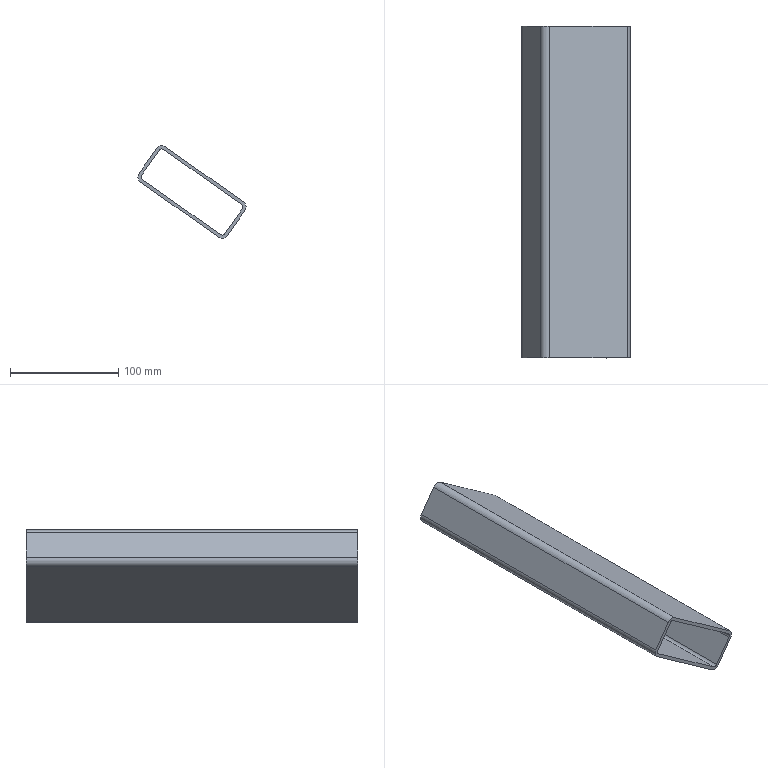Part | STEP file | new extension bracket | 1 solid | 18 faces | box 100.038 x 307.108 x 85.627 mm | volume 239797 mm3 | plane 10 | cylinder 8 | commonest cylinder face diameters 6 x4 12 x4
STEP:
#1=CARTESIAN_POINT('',(0.,0.,0.));
#2=DIRECTION('',(0.,0.,1.));
#3=DIRECTION('',(1.,0.,0.));
#4=AXIS2_PLACEMENT_3D('',#1,#2,#3);
#5=CARTESIAN_POINT('',(1487.978,118.392,730.631));
#6=VERTEX_POINT('',#5);
#7=CARTESIAN_POINT('',(1471.83,118.392,707.757));
#8=VERTEX_POINT('',#7);
#9=CARTESIAN_POINT('',(1489.709,118.392,733.082));
#10=DIRECTION('',(-0.5767,0.,-0.8169));
#11=VECTOR('',#10,1.);
#12=LINE('',#9,#11);
#13=CARTESIAN_POINT('',(0.,118.392,0.));
#14=DIRECTION('',(0.,1.,0.));
#15=DIRECTION('',(0.,0.,-1.));
#16=AXIS2_PLACEMENT_3D('',#13,#14,#15);
#17=PLANE('',#16);
#18=CARTESIAN_POINT('',(-733.082,-1489.709));
#19=DIRECTION('',(0.8169,0.5767));
#20=VECTOR('',#19,1.);
#21=LINE('',#18,#20);
#22=(GEOMETRIC_REPRESENTATION_CONTEXT(2)PARAMETRIC_REPRESENTATION_CONTEXT()REPRESENTATION_CONTEXT('',''));
#23=DEFINITIONAL_REPRESENTATION('',(#21),#22);
#24=PCURVE('',#17,#23);
#25=CARTESIAN_POINT('',(1489.709,425.5,733.082));
#26=DIRECTION('',(-0.8169,0.,0.5767));
#27=DIRECTION('',(-0.5767,0.,-0.8169));
#28=AXIS2_PLACEMENT_3D('',#25,#26,#27);
#29=PLANE('',#28);
#30=CARTESIAN_POINT('',(0.,307.108));
#31=DIRECTION('',(1.,0.));
#32=VECTOR('',#31,1.);
#33=LINE('',#30,#32);
#34=(GEOMETRIC_REPRESENTATION_CONTEXT(2)PARAMETRIC_REPRESENTATION_CONTEXT()REPRESENTATION_CONTEXT('',''));
#35=DEFINITIONAL_REPRESENTATION('',(#33),#34);
#36=PCURVE('',#29,#35);
#37=SURFACE_CURVE('',#12,(#24,#36),.PCURVE_S1.);
#38=EDGE_CURVE('',#6,#8,#37,.T.);
#39=ORIENTED_EDGE('',*,*,#38,.F.);
#40=CARTESIAN_POINT('',(1492.159,118.392,731.351));
#41=VERTEX_POINT('',#40);
#42=CARTESIAN_POINT('',(1490.429,118.392,728.901));
#43=DIRECTION('',(0.,1.,0.));
#44=DIRECTION('',(0.,0.,1.));
#45=AXIS2_PLACEMENT_3D('',#42,#43,#44);
#46=CIRCLE('',#45,3.);
#47=CARTESIAN_POINT('',(-728.901,-1490.429));
#48=DIRECTION('',(-1.,0.));
#49=AXIS2_PLACEMENT_2D('',#47,#48);
#50=CIRCLE('',#49,3.);
#51=(GEOMETRIC_REPRESENTATION_CONTEXT(2)PARAMETRIC_REPRESENTATION_CONTEXT()REPRESENTATION_CONTEXT('',''));
#52=DEFINITIONAL_REPRESENTATION('',(#50),#51);
#53=PCURVE('',#17,#52);
#54=CARTESIAN_POINT('',(1490.429,425.5,728.901));
#55=DIRECTION('',(0.,1.,0.));
#56=DIRECTION('',(1.,0.,0.));
#57=AXIS2_PLACEMENT_3D('',#54,#55,#56);
#58=CYLINDRICAL_SURFACE('',#57,3.);
#59=CARTESIAN_POINT('',(-1.571,-307.108));
#60=DIRECTION('',(1.,0.));
#61=VECTOR('',#60,1.);
#62=LINE('',#59,#61);
#63=(GEOMETRIC_REPRESENTATION_CONTEXT(2)PARAMETRIC_REPRESENTATION_CONTEXT()REPRESENTATION_CONTEXT('',''));
#64=DEFINITIONAL_REPRESENTATION('',(#62),#63);
#65=PCURVE('',#58,#64);
#66=SURFACE_CURVE('',#46,(#53,#65),.PCURVE_S1.);
#67=EDGE_CURVE('',#6,#41,#66,.T.);
#68=ORIENTED_EDGE('',*,*,#67,.T.);
#69=CARTESIAN_POINT('',(1564.049,118.392,680.598));
#70=VERTEX_POINT('',#69);
#71=CARTESIAN_POINT('',(1566.5,118.392,678.868));
#72=DIRECTION('',(-0.8169,0.,0.5767));
#73=VECTOR('',#72,1.);
#74=LINE('',#71,#73);
#75=CARTESIAN_POINT('',(-678.868,-1566.5));
#76=DIRECTION('',(-0.5767,0.8169));
#77=VECTOR('',#76,1.);
#78=LINE('',#75,#77);
#79=(GEOMETRIC_REPRESENTATION_CONTEXT(2)PARAMETRIC_REPRESENTATION_CONTEXT()REPRESENTATION_CONTEXT('',''));
#80=DEFINITIONAL_REPRESENTATION('',(#78),#79);
#81=PCURVE('',#17,#80);
#82=CARTESIAN_POINT('',(1566.5,425.5,678.868));
#83=DIRECTION('',(0.5767,0.,0.8169));
#84=DIRECTION('',(-0.8169,0.,0.5767));
#85=AXIS2_PLACEMENT_3D('',#82,#83,#84);
#86=PLANE('',#85);
#87=CARTESIAN_POINT('',(0.,307.108));
#88=DIRECTION('',(1.,0.));
#89=VECTOR('',#88,1.);
#90=LINE('',#87,#89);
#91=(GEOMETRIC_REPRESENTATION_CONTEXT(2)PARAMETRIC_REPRESENTATION_CONTEXT()REPRESENTATION_CONTEXT('',''));
#92=DEFINITIONAL_REPRESENTATION('',(#90),#91);
#93=PCURVE('',#86,#92);
#94=SURFACE_CURVE('',#74,(#81,#93),.PCURVE_S1.);
#95=EDGE_CURVE('',#70,#41,#94,.T.);
#96=ORIENTED_EDGE('',*,*,#95,.F.);
#97=CARTESIAN_POINT('',(1564.77,118.392,676.417));
#98=VERTEX_POINT('',#97);
#99=CARTESIAN_POINT('',(1562.319,118.392,678.148));
#100=DIRECTION('',(0.,1.,0.));
#101=DIRECTION('',(0.,0.,1.));
#102=AXIS2_PLACEMENT_3D('',#99,#100,#101);
#103=CIRCLE('',#102,3.);
#104=CARTESIAN_POINT('',(-678.148,-1562.319));
#105=DIRECTION('',(-1.,0.));
#106=AXIS2_PLACEMENT_2D('',#104,#105);
#107=CIRCLE('',#106,3.);
#108=(GEOMETRIC_REPRESENTATION_CONTEXT(2)PARAMETRIC_REPRESENTATION_CONTEXT()REPRESENTATION_CONTEXT('',''));
#109=DEFINITIONAL_REPRESENTATION('',(#107),#108);
#110=PCURVE('',#17,#109);
#111=CARTESIAN_POINT('',(1562.319,425.5,678.148));
#112=DIRECTION('',(0.,1.,0.));
#113=DIRECTION('',(1.,0.,0.));
#114=AXIS2_PLACEMENT_3D('',#111,#112,#113);
#115=CYLINDRICAL_SURFACE('',#114,3.);
#116=CARTESIAN_POINT('',(4.712,-307.108));
#117=DIRECTION('',(1.,0.));
#118=VECTOR('',#117,1.);
#119=LINE('',#116,#118);
#120=(GEOMETRIC_REPRESENTATION_CONTEXT(2)PARAMETRIC_REPRESENTATION_CONTEXT()REPRESENTATION_CONTEXT('',''));
#121=DEFINITIONAL_REPRESENTATION('',(#119),#120);
#122=PCURVE('',#115,#121);
#123=SURFACE_CURVE('',#103,(#110,#122),.PCURVE_S1.);
#124=EDGE_CURVE('',#70,#98,#123,.T.);
#125=ORIENTED_EDGE('',*,*,#124,.T.);
#126=CARTESIAN_POINT('',(1548.621,118.392,653.543));
#127=VERTEX_POINT('',#126);
#128=CARTESIAN_POINT('',(1546.891,118.392,651.093));
#129=DIRECTION('',(0.5767,0.,0.8169));
#130=VECTOR('',#129,1.);
#131=LINE('',#128,#130);
#132=CARTESIAN_POINT('',(-651.093,-1546.891));
#133=DIRECTION('',(-0.8169,-0.5767));
#134=VECTOR('',#133,1.);
#135=LINE('',#132,#134);
#136=(GEOMETRIC_REPRESENTATION_CONTEXT(2)PARAMETRIC_REPRESENTATION_CONTEXT()REPRESENTATION_CONTEXT('',''));
#137=DEFINITIONAL_REPRESENTATION('',(#135),#136);
#138=PCURVE('',#17,#137);
#139=CARTESIAN_POINT('',(1546.891,425.5,651.093));
#140=DIRECTION('',(0.8169,0.,-0.5767));
#141=DIRECTION('',(0.5767,0.,0.8169));
#142=AXIS2_PLACEMENT_3D('',#139,#140,#141);
#143=PLANE('',#142);
#144=CARTESIAN_POINT('',(0.,307.108));
#145=DIRECTION('',(1.,0.));
#146=VECTOR('',#145,1.);
#147=LINE('',#144,#146);
#148=(GEOMETRIC_REPRESENTATION_CONTEXT(2)PARAMETRIC_REPRESENTATION_CONTEXT()REPRESENTATION_CONTEXT('',''));
#149=DEFINITIONAL_REPRESENTATION('',(#147),#148);
#150=PCURVE('',#143,#149);
#151=SURFACE_CURVE('',#131,(#138,#150),.PCURVE_S1.);
#152=EDGE_CURVE('',#127,#98,#151,.T.);
#153=ORIENTED_EDGE('',*,*,#152,.F.);
#154=CARTESIAN_POINT('',(1544.44,118.392,652.823));
#155=VERTEX_POINT('',#154);
#156=CARTESIAN_POINT('',(1546.17,118.392,655.274));
#157=DIRECTION('',(0.,1.,0.));
#158=DIRECTION('',(0.,0.,1.));
#159=AXIS2_PLACEMENT_3D('',#156,#157,#158);
#160=CIRCLE('',#159,3.);
#161=CARTESIAN_POINT('',(-655.274,-1546.17));
#162=DIRECTION('',(-1.,0.));
#163=AXIS2_PLACEMENT_2D('',#161,#162);
#164=CIRCLE('',#163,3.);
#165=(GEOMETRIC_REPRESENTATION_CONTEXT(2)PARAMETRIC_REPRESENTATION_CONTEXT()REPRESENTATION_CONTEXT('',''));
#166=DEFINITIONAL_REPRESENTATION('',(#164),#165);
#167=PCURVE('',#17,#166);
#168=CARTESIAN_POINT('',(1546.17,425.5,655.274));
#169=DIRECTION('',(0.,1.,0.));
#170=DIRECTION('',(1.,0.,0.));
#171=AXIS2_PLACEMENT_3D('',#168,#169,#170);
#172=CYLINDRICAL_SURFACE('',#171,3.);
#173=CARTESIAN_POINT('',(-1.571,-307.108));
#174=DIRECTION('',(1.,0.));
#175=VECTOR('',#174,1.);
#176=LINE('',#173,#175);
#177=(GEOMETRIC_REPRESENTATION_CONTEXT(2)PARAMETRIC_REPRESENTATION_CONTEXT()REPRESENTATION_CONTEXT('',''));
#178=DEFINITIONAL_REPRESENTATION('',(#176),#177);
#179=PCURVE('',#172,#178);
#180=SURFACE_CURVE('',#160,(#167,#179),.PCURVE_S1.);
#181=EDGE_CURVE('',#127,#155,#180,.T.);
#182=ORIENTED_EDGE('',*,*,#181,.T.);
#183=CARTESIAN_POINT('',(1472.55,118.392,703.576));
#184=VERTEX_POINT('',#183);
#185=CARTESIAN_POINT('',(1470.099,118.392,705.306));
#186=DIRECTION('',(0.8169,0.,-0.5767));
#187=VECTOR('',#186,1.);
#188=LINE('',#185,#187);
#189=CARTESIAN_POINT('',(-705.306,-1470.099));
#190=DIRECTION('',(0.5767,-0.8169));
#191=VECTOR('',#190,1.);
#192=LINE('',#189,#191);
#193=(GEOMETRIC_REPRESENTATION_CONTEXT(2)PARAMETRIC_REPRESENTATION_CONTEXT()REPRESENTATION_CONTEXT('',''));
#194=DEFINITIONAL_REPRESENTATION('',(#192),#193);
#195=PCURVE('',#17,#194);
#196=CARTESIAN_POINT('',(1470.099,425.5,705.306));
#197=DIRECTION('',(-0.5767,0.,-0.8169));
#198=DIRECTION('',(0.8169,0.,-0.5767));
#199=AXIS2_PLACEMENT_3D('',#196,#197,#198);
#200=PLANE('',#199);
#201=CARTESIAN_POINT('',(0.,307.108));
#202=DIRECTION('',(1.,0.));
#203=VECTOR('',#202,1.);
#204=LINE('',#201,#203);
#205=(GEOMETRIC_REPRESENTATION_CONTEXT(2)PARAMETRIC_REPRESENTATION_CONTEXT()REPRESENTATION_CONTEXT('',''));
#206=DEFINITIONAL_REPRESENTATION('',(#204),#205);
#207=PCURVE('',#200,#206);
#208=SURFACE_CURVE('',#188,(#195,#207),.PCURVE_S1.);
#209=EDGE_CURVE('',#184,#155,#208,.T.);
#210=ORIENTED_EDGE('',*,*,#209,.F.);
#211=CARTESIAN_POINT('',(1474.28,118.392,706.027));
#212=DIRECTION('',(0.,1.,0.));
#213=DIRECTION('',(0.,0.,1.));
#214=AXIS2_PLACEMENT_3D('',#211,#212,#213);
#215=CIRCLE('',#214,3.);
#216=CARTESIAN_POINT('',(-706.027,-1474.28));
#217=DIRECTION('',(-1.,0.));
#218=AXIS2_PLACEMENT_2D('',#216,#217);
#219=CIRCLE('',#218,3.);
#220=(GEOMETRIC_REPRESENTATION_CONTEXT(2)PARAMETRIC_REPRESENTATION_CONTEXT()REPRESENTATION_CONTEXT('',''));
#221=DEFINITIONAL_REPRESENTATION('',(#219),#220);
#222=PCURVE('',#17,#221);
#223=CARTESIAN_POINT('',(1474.28,425.5,706.027));
#224=DIRECTION('',(0.,1.,0.));
#225=DIRECTION('',(1.,0.,0.));
#226=AXIS2_PLACEMENT_3D('',#223,#224,#225);
#227=CYLINDRICAL_SURFACE('',#226,3.);
#228=CARTESIAN_POINT('',(-1.571,-307.108));
#229=DIRECTION('',(1.,0.));
#230=VECTOR('',#229,1.);
#231=LINE('',#228,#230);
#232=(GEOMETRIC_REPRESENTATION_CONTEXT(2)PARAMETRIC_REPRESENTATION_CONTEXT()REPRESENTATION_CONTEXT('',''));
#233=DEFINITIONAL_REPRESENTATION('',(#231),#232);
#234=PCURVE('',#227,#233);
#235=SURFACE_CURVE('',#215,(#222,#234),.PCURVE_S1.);
#236=EDGE_CURVE('',#184,#8,#235,.T.);
#237=ORIENTED_EDGE('',*,*,#236,.T.);
#238=EDGE_LOOP('',(#39,#68,#96,#125,#153,#182,#210,#237));
#239=FACE_BOUND('',#238,.T.);
#240=CARTESIAN_POINT('',(1542.71,118.392,650.372));
#241=VERTEX_POINT('',#240);
#242=CARTESIAN_POINT('',(1470.82,118.392,701.125));
#243=VERTEX_POINT('',#242);
#244=CARTESIAN_POINT('',(1547.611,118.392,646.912));
#245=DIRECTION('',(-0.8169,0.,0.5767));
#246=VECTOR('',#245,1.);
#247=LINE('',#244,#246);
#248=CARTESIAN_POINT('',(-646.912,-1547.611));
#249=DIRECTION('',(-0.5767,0.8169));
#250=VECTOR('',#249,1.);
#251=LINE('',#248,#250);
#252=(GEOMETRIC_REPRESENTATION_CONTEXT(2)PARAMETRIC_REPRESENTATION_CONTEXT()REPRESENTATION_CONTEXT('',''));
#253=DEFINITIONAL_REPRESENTATION('',(#251),#252);
#254=PCURVE('',#17,#253);
#255=CARTESIAN_POINT('',(1547.611,425.5,646.912));
#256=DIRECTION('',(0.5767,0.,0.8169));
#257=DIRECTION('',(-0.8169,0.,0.5767));
#258=AXIS2_PLACEMENT_3D('',#255,#256,#257);
#259=PLANE('',#258);
#260=CARTESIAN_POINT('',(0.,307.108));
#261=DIRECTION('',(1.,0.));
#262=VECTOR('',#261,1.);
#263=LINE('',#260,#262);
#264=(GEOMETRIC_REPRESENTATION_CONTEXT(2)PARAMETRIC_REPRESENTATION_CONTEXT()REPRESENTATION_CONTEXT('',''));
#265=DEFINITIONAL_REPRESENTATION('',(#263),#264);
#266=PCURVE('',#259,#265);
#267=SURFACE_CURVE('',#247,(#254,#266),.PCURVE_S1.);
#268=EDGE_CURVE('',#241,#243,#267,.T.);
#269=ORIENTED_EDGE('',*,*,#268,.F.);
#270=CARTESIAN_POINT('',(1551.072,118.392,651.813));
#271=VERTEX_POINT('',#270);
#272=CARTESIAN_POINT('',(1546.17,118.392,655.274));
#273=DIRECTION('',(0.,-1.,0.));
#274=DIRECTION('',(0.,0.,1.));
#275=AXIS2_PLACEMENT_3D('',#272,#273,#274);
#276=CIRCLE('',#275,6.);
#277=CARTESIAN_POINT('',(-661.274,-1546.17));
#278=CARTESIAN_POINT('',(-661.274,-1535.778));
#279=CARTESIAN_POINT('',(-652.274,-1540.974));
#280=CARTESIAN_POINT('',(-643.274,-1546.17));
#281=CARTESIAN_POINT('',(-652.274,-1551.366));
#282=CARTESIAN_POINT('',(-661.274,-1556.562));
#283=CARTESIAN_POINT('',(-661.274,-1546.17));
#284=(BOUNDED_CURVE()B_SPLINE_CURVE(2,(#277,#278,#279,#280,#281,#282,#283),.UNSPECIFIED.,.T.,.F.)B_SPLINE_CURVE_WITH_KNOTS((1,2,2,2,2,1),(-2.094,0.,2.094,4.189,6.283,8.378),.UNSPECIFIED.)CURVE()GEOMETRIC_REPRESENTATION_ITEM()RATIONAL_B_SPLINE_CURVE((1.,0.5,1.,0.5,1.,0.5,1.))REPRESENTATION_ITEM(''));
#285=(GEOMETRIC_REPRESENTATION_CONTEXT(2)PARAMETRIC_REPRESENTATION_CONTEXT()REPRESENTATION_CONTEXT('',''));
#286=DEFINITIONAL_REPRESENTATION('',(#284),#285);
#287=PCURVE('',#17,#286);
#288=CARTESIAN_POINT('',(1546.17,425.5,655.274));
#289=DIRECTION('',(0.,-1.,0.));
#290=DIRECTION('',(-1.,0.,0.));
#291=AXIS2_PLACEMENT_3D('',#288,#289,#290);
#292=CYLINDRICAL_SURFACE('',#291,6.);
#293=CARTESIAN_POINT('',(-1.571,307.108));
#294=DIRECTION('',(1.,0.));
#295=VECTOR('',#294,1.);
#296=LINE('',#293,#295);
#297=(GEOMETRIC_REPRESENTATION_CONTEXT(2)PARAMETRIC_REPRESENTATION_CONTEXT()REPRESENTATION_CONTEXT('',''));
#298=DEFINITIONAL_REPRESENTATION('',(#296),#297);
#299=PCURVE('',#292,#298);
#300=SURFACE_CURVE('',#276,(#287,#299),.PCURVE_S1.);
#301=EDGE_CURVE('',#241,#271,#300,.T.);
#302=ORIENTED_EDGE('',*,*,#301,.T.);
#303=CARTESIAN_POINT('',(1567.22,118.392,674.687));
#304=VERTEX_POINT('',#303);
#305=CARTESIAN_POINT('',(1570.681,118.392,679.589));
#306=DIRECTION('',(-0.5767,0.,-0.8169));
#307=VECTOR('',#306,1.);
#308=LINE('',#305,#307);
#309=CARTESIAN_POINT('',(-679.589,-1570.681));
#310=DIRECTION('',(0.8169,0.5767));
#311=VECTOR('',#310,1.);
#312=LINE('',#309,#311);
#313=(GEOMETRIC_REPRESENTATION_CONTEXT(2)PARAMETRIC_REPRESENTATION_CONTEXT()REPRESENTATION_CONTEXT('',''));
#314=DEFINITIONAL_REPRESENTATION('',(#312),#313);
#315=PCURVE('',#17,#314);
#316=CARTESIAN_POINT('',(1570.681,425.5,679.589));
#317=DIRECTION('',(-0.8169,0.,0.5767));
#318=DIRECTION('',(-0.5767,0.,-0.8169));
#319=AXIS2_PLACEMENT_3D('',#316,#317,#318);
#320=PLANE('',#319);
#321=CARTESIAN_POINT('',(0.,307.108));
#322=DIRECTION('',(1.,0.));
#323=VECTOR('',#322,1.);
#324=LINE('',#321,#323);
#325=(GEOMETRIC_REPRESENTATION_CONTEXT(2)PARAMETRIC_REPRESENTATION_CONTEXT()REPRESENTATION_CONTEXT('',''));
#326=DEFINITIONAL_REPRESENTATION('',(#324),#325);
#327=PCURVE('',#320,#326);
#328=SURFACE_CURVE('',#308,(#315,#327),.PCURVE_S1.);
#329=EDGE_CURVE('',#304,#271,#328,.T.);
#330=ORIENTED_EDGE('',*,*,#329,.F.);
#331=CARTESIAN_POINT('',(1565.779,118.392,683.049));
#332=VERTEX_POINT('',#331);
#333=CARTESIAN_POINT('',(1562.319,118.392,678.148));
#334=DIRECTION('',(0.,-1.,0.));
#335=DIRECTION('',(0.,0.,1.));
#336=AXIS2_PLACEMENT_3D('',#333,#334,#335);
#337=CIRCLE('',#336,6.);
#338=CARTESIAN_POINT('',(-684.148,-1562.319));
#339=CARTESIAN_POINT('',(-684.148,-1551.927));
#340=CARTESIAN_POINT('',(-675.148,-1557.123));
#341=CARTESIAN_POINT('',(-666.148,-1562.319));
#342=CARTESIAN_POINT('',(-675.148,-1567.515));
#343=CARTESIAN_POINT('',(-684.148,-1572.711));
#344=CARTESIAN_POINT('',(-684.148,-1562.319));
#345=(BOUNDED_CURVE()B_SPLINE_CURVE(2,(#338,#339,#340,#341,#342,#343,#344),.UNSPECIFIED.,.T.,.F.)B_SPLINE_CURVE_WITH_KNOTS((1,2,2,2,2,1),(-2.094,0.,2.094,4.189,6.283,8.378),.UNSPECIFIED.)CURVE()GEOMETRIC_REPRESENTATION_ITEM()RATIONAL_B_SPLINE_CURVE((1.,0.5,1.,0.5,1.,0.5,1.))REPRESENTATION_ITEM(''));
#346=(GEOMETRIC_REPRESENTATION_CONTEXT(2)PARAMETRIC_REPRESENTATION_CONTEXT()REPRESENTATION_CONTEXT('',''));
#347=DEFINITIONAL_REPRESENTATION('',(#345),#346);
#348=PCURVE('',#17,#347);
#349=CARTESIAN_POINT('',(1562.319,425.5,678.148));
#350=DIRECTION('',(0.,-1.,0.));
#351=DIRECTION('',(-1.,0.,0.));
#352=AXIS2_PLACEMENT_3D('',#349,#350,#351);
#353=CYLINDRICAL_SURFACE('',#352,6.);
#354=CARTESIAN_POINT('',(-1.571,307.108));
#355=DIRECTION('',(1.,0.));
#356=VECTOR('',#355,1.);
#357=LINE('',#354,#356);
#358=(GEOMETRIC_REPRESENTATION_CONTEXT(2)PARAMETRIC_REPRESENTATION_CONTEXT()REPRESENTATION_CONTEXT('',''));
#359=DEFINITIONAL_REPRESENTATION('',(#357),#358);
#360=PCURVE('',#353,#359);
#361=SURFACE_CURVE('',#337,(#348,#360),.PCURVE_S1.);
#362=EDGE_CURVE('',#304,#332,#361,.T.);
#363=ORIENTED_EDGE('',*,*,#362,.T.);
#364=CARTESIAN_POINT('',(1493.89,118.392,733.802));
#365=VERTEX_POINT('',#364);
#366=CARTESIAN_POINT('',(1488.988,118.392,737.263));
#367=DIRECTION('',(0.8169,0.,-0.5767));
#368=VECTOR('',#367,1.);
#369=LINE('',#366,#368);
#370=CARTESIAN_POINT('',(-737.263,-1488.988));
#371=DIRECTION('',(0.5767,-0.8169));
#372=VECTOR('',#371,1.);
#373=LINE('',#370,#372);
#374=(GEOMETRIC_REPRESENTATION_CONTEXT(2)PARAMETRIC_REPRESENTATION_CONTEXT()REPRESENTATION_CONTEXT('',''));
#375=DEFINITIONAL_REPRESENTATION('',(#373),#374);
#376=PCURVE('',#17,#375);
#377=CARTESIAN_POINT('',(1488.988,425.5,737.263));
#378=DIRECTION('',(-0.5767,0.,-0.8169));
#379=DIRECTION('',(0.8169,0.,-0.5767));
#380=AXIS2_PLACEMENT_3D('',#377,#378,#379);
#381=PLANE('',#380);
#382=CARTESIAN_POINT('',(0.,307.108));
#383=DIRECTION('',(1.,0.));
#384=VECTOR('',#383,1.);
#385=LINE('',#382,#384);
#386=(GEOMETRIC_REPRESENTATION_CONTEXT(2)PARAMETRIC_REPRESENTATION_CONTEXT()REPRESENTATION_CONTEXT('',''));
#387=DEFINITIONAL_REPRESENTATION('',(#385),#386);
#388=PCURVE('',#381,#387);
#389=SURFACE_CURVE('',#369,(#376,#388),.PCURVE_S1.);
#390=EDGE_CURVE('',#365,#332,#389,.T.);
#391=ORIENTED_EDGE('',*,*,#390,.F.);
#392=CARTESIAN_POINT('',(1485.528,118.392,732.361));
#393=VERTEX_POINT('',#392);
#394=CARTESIAN_POINT('',(1490.429,118.392,728.901));
#395=DIRECTION('',(0.,-1.,0.));
#396=DIRECTION('',(0.,0.,1.));
#397=AXIS2_PLACEMENT_3D('',#394,#395,#396);
#398=CIRCLE('',#397,6.);
#399=CARTESIAN_POINT('',(-734.901,-1490.429));
#400=CARTESIAN_POINT('',(-734.901,-1480.037));
#401=CARTESIAN_POINT('',(-725.901,-1485.233));
#402=CARTESIAN_POINT('',(-716.901,-1490.429));
#403=CARTESIAN_POINT('',(-725.901,-1495.625));
#404=CARTESIAN_POINT('',(-734.901,-1500.821));
#405=CARTESIAN_POINT('',(-734.901,-1490.429));
#406=(BOUNDED_CURVE()B_SPLINE_CURVE(2,(#399,#400,#401,#402,#403,#404,#405),.UNSPECIFIED.,.T.,.F.)B_SPLINE_CURVE_WITH_KNOTS((1,2,2,2,2,1),(-2.094,0.,2.094,4.189,6.283,8.378),.UNSPECIFIED.)CURVE()GEOMETRIC_REPRESENTATION_ITEM()RATIONAL_B_SPLINE_CURVE((1.,0.5,1.,0.5,1.,0.5,1.))REPRESENTATION_ITEM(''));
#407=(GEOMETRIC_REPRESENTATION_CONTEXT(2)PARAMETRIC_REPRESENTATION_CONTEXT()REPRESENTATION_CONTEXT('',''));
#408=DEFINITIONAL_REPRESENTATION('',(#406),#407);
#409=PCURVE('',#17,#408);
#410=CARTESIAN_POINT('',(1490.429,425.5,728.901));
#411=DIRECTION('',(0.,-1.,0.));
#412=DIRECTION('',(-1.,0.,0.));
#413=AXIS2_PLACEMENT_3D('',#410,#411,#412);
#414=CYLINDRICAL_SURFACE('',#413,6.);
#415=CARTESIAN_POINT('',(-1.571,307.108));
#416=DIRECTION('',(1.,0.));
#417=VECTOR('',#416,1.);
#418=LINE('',#415,#417);
#419=(GEOMETRIC_REPRESENTATION_CONTEXT(2)PARAMETRIC_REPRESENTATION_CONTEXT()REPRESENTATION_CONTEXT('',''));
#420=DEFINITIONAL_REPRESENTATION('',(#418),#419);
#421=PCURVE('',#414,#420);
#422=SURFACE_CURVE('',#398,(#409,#421),.PCURVE_S1.);
#423=EDGE_CURVE('',#365,#393,#422,.T.);
#424=ORIENTED_EDGE('',*,*,#423,.T.);
#425=CARTESIAN_POINT('',(1469.379,118.392,709.487));
#426=VERTEX_POINT('',#425);
#427=CARTESIAN_POINT('',(1465.918,118.392,704.586));
#428=DIRECTION('',(0.5767,0.,0.8169));
#429=VECTOR('',#428,1.);
#430=LINE('',#427,#429);
#431=CARTESIAN_POINT('',(-704.586,-1465.918));
#432=DIRECTION('',(-0.8169,-0.5767));
#433=VECTOR('',#432,1.);
#434=LINE('',#431,#433);
#435=(GEOMETRIC_REPRESENTATION_CONTEXT(2)PARAMETRIC_REPRESENTATION_CONTEXT()REPRESENTATION_CONTEXT('',''));
#436=DEFINITIONAL_REPRESENTATION('',(#434),#435);
#437=PCURVE('',#17,#436);
#438=CARTESIAN_POINT('',(1465.918,425.5,704.586));
#439=DIRECTION('',(0.8169,0.,-0.5767));
#440=DIRECTION('',(0.5767,0.,0.8169));
#441=AXIS2_PLACEMENT_3D('',#438,#439,#440);
#442=PLANE('',#441);
#443=CARTESIAN_POINT('',(0.,307.108));
#444=DIRECTION('',(1.,0.));
#445=VECTOR('',#444,1.);
#446=LINE('',#443,#445);
#447=(GEOMETRIC_REPRESENTATION_CONTEXT(2)PARAMETRIC_REPRESENTATION_CONTEXT()REPRESENTATION_CONTEXT('',''));
#448=DEFINITIONAL_REPRESENTATION('',(#446),#447);
#449=PCURVE('',#442,#448);
#450=SURFACE_CURVE('',#430,(#437,#449),.PCURVE_S1.);
#451=EDGE_CURVE('',#426,#393,#450,.T.);
#452=ORIENTED_EDGE('',*,*,#451,.F.);
#453=CARTESIAN_POINT('',(1474.28,118.392,706.027));
#454=DIRECTION('',(0.,-1.,0.));
#455=DIRECTION('',(0.,0.,1.));
#456=AXIS2_PLACEMENT_3D('',#453,#454,#455);
#457=CIRCLE('',#456,6.);
#458=CARTESIAN_POINT('',(-712.027,-1474.28));
#459=CARTESIAN_POINT('',(-712.027,-1463.888));
#460=CARTESIAN_POINT('',(-703.027,-1469.084));
#461=CARTESIAN_POINT('',(-694.027,-1474.28));
#462=CARTESIAN_POINT('',(-703.027,-1479.477));
#463=CARTESIAN_POINT('',(-712.027,-1484.673));
#464=CARTESIAN_POINT('',(-712.027,-1474.28));
#465=(BOUNDED_CURVE()B_SPLINE_CURVE(2,(#458,#459,#460,#461,#462,#463,#464),.UNSPECIFIED.,.T.,.F.)B_SPLINE_CURVE_WITH_KNOTS((1,2,2,2,2,1),(-2.094,0.,2.094,4.189,6.283,8.378),.UNSPECIFIED.)CURVE()GEOMETRIC_REPRESENTATION_ITEM()RATIONAL_B_SPLINE_CURVE((1.,0.5,1.,0.5,1.,0.5,1.))REPRESENTATION_ITEM(''));
#466=(GEOMETRIC_REPRESENTATION_CONTEXT(2)PARAMETRIC_REPRESENTATION_CONTEXT()REPRESENTATION_CONTEXT('',''));
#467=DEFINITIONAL_REPRESENTATION('',(#465),#466);
#468=PCURVE('',#17,#467);
#469=CARTESIAN_POINT('',(1474.28,425.5,706.027));
#470=DIRECTION('',(0.,-1.,0.));
#471=DIRECTION('',(-1.,0.,0.));
#472=AXIS2_PLACEMENT_3D('',#469,#470,#471);
#473=CYLINDRICAL_SURFACE('',#472,6.);
#474=CARTESIAN_POINT('',(-1.571,307.108));
#475=DIRECTION('',(1.,0.));
#476=VECTOR('',#475,1.);
#477=LINE('',#474,#476);
#478=(GEOMETRIC_REPRESENTATION_CONTEXT(2)PARAMETRIC_REPRESENTATION_CONTEXT()REPRESENTATION_CONTEXT('',''));
#479=DEFINITIONAL_REPRESENTATION('',(#477),#478);
#480=PCURVE('',#473,#479);
#481=SURFACE_CURVE('',#457,(#468,#480),.PCURVE_S1.);
#482=EDGE_CURVE('',#426,#243,#481,.T.);
#483=ORIENTED_EDGE('',*,*,#482,.T.);
#484=EDGE_LOOP('',(#269,#302,#330,#363,#391,#424,#452,#483));
#485=FACE_BOUND('',#484,.T.);
#486=ADVANCED_FACE('',(#239,#485),#17,.F.);
#487=CARTESIAN_POINT('',(1548.621,425.5,653.543));
#488=VERTEX_POINT('',#487);
#489=CARTESIAN_POINT('',(1564.77,425.5,676.417));
#490=VERTEX_POINT('',#489);
#491=CARTESIAN_POINT('',(1546.891,425.5,651.093));
#492=DIRECTION('',(0.5767,0.,0.8169));
#493=VECTOR('',#492,1.);
#494=LINE('',#491,#493);
#495=CARTESIAN_POINT('',(0.,425.5,0.));
#496=DIRECTION('',(0.,1.,0.));
#497=DIRECTION('',(0.,0.,-1.));
#498=AXIS2_PLACEMENT_3D('',#495,#496,#497);
#499=PLANE('',#498);
#500=CARTESIAN_POINT('',(-651.093,-1546.891));
#501=DIRECTION('',(-0.8169,-0.5767));
#502=VECTOR('',#501,1.);
#503=LINE('',#500,#502);
#504=(GEOMETRIC_REPRESENTATION_CONTEXT(2)PARAMETRIC_REPRESENTATION_CONTEXT()REPRESENTATION_CONTEXT('',''));
#505=DEFINITIONAL_REPRESENTATION('',(#503),#504);
#506=PCURVE('',#499,#505);
#507=CARTESIAN_POINT('',(0.,0.));
#508=DIRECTION('',(1.,0.));
#509=VECTOR('',#508,1.);
#510=LINE('',#507,#509);
#511=(GEOMETRIC_REPRESENTATION_CONTEXT(2)PARAMETRIC_REPRESENTATION_CONTEXT()REPRESENTATION_CONTEXT('',''));
#512=DEFINITIONAL_REPRESENTATION('',(#510),#511);
#513=PCURVE('',#143,#512);
#514=SURFACE_CURVE('',#494,(#506,#513),.PCURVE_S1.);
#515=EDGE_CURVE('',#488,#490,#514,.T.);
#516=ORIENTED_EDGE('',*,*,#515,.T.);
#517=CARTESIAN_POINT('',(1564.049,425.5,680.598));
#518=VERTEX_POINT('',#517);
#519=CARTESIAN_POINT('',(1562.319,425.5,678.148));
#520=DIRECTION('',(0.,-1.,0.));
#521=DIRECTION('',(0.,0.,1.));
#522=AXIS2_PLACEMENT_3D('',#519,#520,#521);
#523=CIRCLE('',#522,3.);
#524=CARTESIAN_POINT('',(-681.148,-1562.319));
#525=CARTESIAN_POINT('',(-681.148,-1557.123));
#526=CARTESIAN_POINT('',(-676.648,-1559.721));
#527=CARTESIAN_POINT('',(-672.148,-1562.319));
#528=CARTESIAN_POINT('',(-676.648,-1564.917));
#529=CARTESIAN_POINT('',(-681.148,-1567.515));
#530=CARTESIAN_POINT('',(-681.148,-1562.319));
#531=(BOUNDED_CURVE()B_SPLINE_CURVE(2,(#524,#525,#526,#527,#528,#529,#530),.UNSPECIFIED.,.T.,.F.)B_SPLINE_CURVE_WITH_KNOTS((1,2,2,2,2,1),(-2.094,0.,2.094,4.189,6.283,8.378),.UNSPECIFIED.)CURVE()GEOMETRIC_REPRESENTATION_ITEM()RATIONAL_B_SPLINE_CURVE((1.,0.5,1.,0.5,1.,0.5,1.))REPRESENTATION_ITEM(''));
#532=(GEOMETRIC_REPRESENTATION_CONTEXT(2)PARAMETRIC_REPRESENTATION_CONTEXT()REPRESENTATION_CONTEXT('',''));
#533=DEFINITIONAL_REPRESENTATION('',(#531),#532);
#534=PCURVE('',#499,#533);
#535=CARTESIAN_POINT('',(10.996,0.));
#536=DIRECTION('',(-1.,0.));
#537=VECTOR('',#536,1.);
#538=LINE('',#535,#537);
#539=(GEOMETRIC_REPRESENTATION_CONTEXT(2)PARAMETRIC_REPRESENTATION_CONTEXT()REPRESENTATION_CONTEXT('',''));
#540=DEFINITIONAL_REPRESENTATION('',(#538),#539);
#541=PCURVE('',#115,#540);
#542=SURFACE_CURVE('',#523,(#534,#541),.PCURVE_S1.);
#543=EDGE_CURVE('',#490,#518,#542,.T.);
#544=ORIENTED_EDGE('',*,*,#543,.T.);
#545=CARTESIAN_POINT('',(1492.159,425.5,731.351));
#546=VERTEX_POINT('',#545);
#547=CARTESIAN_POINT('',(1566.5,425.5,678.868));
#548=DIRECTION('',(-0.8169,0.,0.5767));
#549=VECTOR('',#548,1.);
#550=LINE('',#547,#549);
#551=CARTESIAN_POINT('',(-678.868,-1566.5));
#552=DIRECTION('',(-0.5767,0.8169));
#553=VECTOR('',#552,1.);
#554=LINE('',#551,#553);
#555=(GEOMETRIC_REPRESENTATION_CONTEXT(2)PARAMETRIC_REPRESENTATION_CONTEXT()REPRESENTATION_CONTEXT('',''));
#556=DEFINITIONAL_REPRESENTATION('',(#554),#555);
#557=PCURVE('',#499,#556);
#558=CARTESIAN_POINT('',(0.,0.));
#559=DIRECTION('',(1.,0.));
#560=VECTOR('',#559,1.);
#561=LINE('',#558,#560);
#562=(GEOMETRIC_REPRESENTATION_CONTEXT(2)PARAMETRIC_REPRESENTATION_CONTEXT()REPRESENTATION_CONTEXT('',''));
#563=DEFINITIONAL_REPRESENTATION('',(#561),#562);
#564=PCURVE('',#86,#563);
#565=SURFACE_CURVE('',#550,(#557,#564),.PCURVE_S1.);
#566=EDGE_CURVE('',#518,#546,#565,.T.);
#567=ORIENTED_EDGE('',*,*,#566,.T.);
#568=CARTESIAN_POINT('',(1487.978,425.5,730.631));
#569=VERTEX_POINT('',#568);
#570=CARTESIAN_POINT('',(1490.429,425.5,728.901));
#571=DIRECTION('',(0.,-1.,0.));
#572=DIRECTION('',(0.,0.,1.));
#573=AXIS2_PLACEMENT_3D('',#570,#571,#572);
#574=CIRCLE('',#573,3.);
#575=CARTESIAN_POINT('',(-731.901,-1490.429));
#576=CARTESIAN_POINT('',(-731.901,-1485.233));
#577=CARTESIAN_POINT('',(-727.401,-1487.831));
#578=CARTESIAN_POINT('',(-722.901,-1490.429));
#579=CARTESIAN_POINT('',(-727.401,-1493.027));
#580=CARTESIAN_POINT('',(-731.901,-1495.625));
#581=CARTESIAN_POINT('',(-731.901,-1490.429));
#582=(BOUNDED_CURVE()B_SPLINE_CURVE(2,(#575,#576,#577,#578,#579,#580,#581),.UNSPECIFIED.,.T.,.F.)B_SPLINE_CURVE_WITH_KNOTS((1,2,2,2,2,1),(-2.094,0.,2.094,4.189,6.283,8.378),.UNSPECIFIED.)CURVE()GEOMETRIC_REPRESENTATION_ITEM()RATIONAL_B_SPLINE_CURVE((1.,0.5,1.,0.5,1.,0.5,1.))REPRESENTATION_ITEM(''));
#583=(GEOMETRIC_REPRESENTATION_CONTEXT(2)PARAMETRIC_REPRESENTATION_CONTEXT()REPRESENTATION_CONTEXT('',''));
#584=DEFINITIONAL_REPRESENTATION('',(#582),#583);
#585=PCURVE('',#499,#584);
#586=CARTESIAN_POINT('',(10.996,0.));
#587=DIRECTION('',(-1.,0.));
#588=VECTOR('',#587,1.);
#589=LINE('',#586,#588);
#590=(GEOMETRIC_REPRESENTATION_CONTEXT(2)PARAMETRIC_REPRESENTATION_CONTEXT()REPRESENTATION_CONTEXT('',''));
#591=DEFINITIONAL_REPRESENTATION('',(#589),#590);
#592=PCURVE('',#58,#591);
#593=SURFACE_CURVE('',#574,(#585,#592),.PCURVE_S1.);
#594=EDGE_CURVE('',#546,#569,#593,.T.);
#595=ORIENTED_EDGE('',*,*,#594,.T.);
#596=CARTESIAN_POINT('',(1471.83,425.5,707.757));
#597=VERTEX_POINT('',#596);
#598=CARTESIAN_POINT('',(1489.709,425.5,733.082));
#599=DIRECTION('',(-0.5767,0.,-0.8169));
#600=VECTOR('',#599,1.);
#601=LINE('',#598,#600);
#602=CARTESIAN_POINT('',(-733.082,-1489.709));
#603=DIRECTION('',(0.8169,0.5767));
#604=VECTOR('',#603,1.);
#605=LINE('',#602,#604);
#606=(GEOMETRIC_REPRESENTATION_CONTEXT(2)PARAMETRIC_REPRESENTATION_CONTEXT()REPRESENTATION_CONTEXT('',''));
#607=DEFINITIONAL_REPRESENTATION('',(#605),#606);
#608=PCURVE('',#499,#607);
#609=CARTESIAN_POINT('',(0.,0.));
#610=DIRECTION('',(1.,0.));
#611=VECTOR('',#610,1.);
#612=LINE('',#609,#611);
#613=(GEOMETRIC_REPRESENTATION_CONTEXT(2)PARAMETRIC_REPRESENTATION_CONTEXT()REPRESENTATION_CONTEXT('',''));
#614=DEFINITIONAL_REPRESENTATION('',(#612),#613);
#615=PCURVE('',#29,#614);
#616=SURFACE_CURVE('',#601,(#608,#615),.PCURVE_S1.);
#617=EDGE_CURVE('',#569,#597,#616,.T.);
#618=ORIENTED_EDGE('',*,*,#617,.T.);
#619=CARTESIAN_POINT('',(1472.55,425.5,703.576));
#620=VERTEX_POINT('',#619);
#621=CARTESIAN_POINT('',(1474.28,425.5,706.027));
#622=DIRECTION('',(0.,-1.,0.));
#623=DIRECTION('',(0.,0.,1.));
#624=AXIS2_PLACEMENT_3D('',#621,#622,#623);
#625=CIRCLE('',#624,3.);
#626=CARTESIAN_POINT('',(-709.027,-1474.28));
#627=CARTESIAN_POINT('',(-709.027,-1469.084));
#628=CARTESIAN_POINT('',(-704.527,-1471.682));
#629=CARTESIAN_POINT('',(-700.027,-1474.28));
#630=CARTESIAN_POINT('',(-704.527,-1476.879));
#631=CARTESIAN_POINT('',(-709.027,-1479.477));
#632=CARTESIAN_POINT('',(-709.027,-1474.28));
#633=(BOUNDED_CURVE()B_SPLINE_CURVE(2,(#626,#627,#628,#629,#630,#631,#632),.UNSPECIFIED.,.T.,.F.)B_SPLINE_CURVE_WITH_KNOTS((1,2,2,2,2,1),(-2.094,0.,2.094,4.189,6.283,8.378),.UNSPECIFIED.)CURVE()GEOMETRIC_REPRESENTATION_ITEM()RATIONAL_B_SPLINE_CURVE((1.,0.5,1.,0.5,1.,0.5,1.))REPRESENTATION_ITEM(''));
#634=(GEOMETRIC_REPRESENTATION_CONTEXT(2)PARAMETRIC_REPRESENTATION_CONTEXT()REPRESENTATION_CONTEXT('',''));
#635=DEFINITIONAL_REPRESENTATION('',(#633),#634);
#636=PCURVE('',#499,#635);
#637=CARTESIAN_POINT('',(4.712,0.));
#638=DIRECTION('',(-1.,0.));
#639=VECTOR('',#638,1.);
#640=LINE('',#637,#639);
#641=(GEOMETRIC_REPRESENTATION_CONTEXT(2)PARAMETRIC_REPRESENTATION_CONTEXT()REPRESENTATION_CONTEXT('',''));
#642=DEFINITIONAL_REPRESENTATION('',(#640),#641);
#643=PCURVE('',#227,#642);
#644=SURFACE_CURVE('',#625,(#636,#643),.PCURVE_S1.);
#645=EDGE_CURVE('',#597,#620,#644,.T.);
#646=ORIENTED_EDGE('',*,*,#645,.T.);
#647=CARTESIAN_POINT('',(1544.44,425.5,652.823));
#648=VERTEX_POINT('',#647);
#649=CARTESIAN_POINT('',(1470.099,425.5,705.306));
#650=DIRECTION('',(0.8169,0.,-0.5767));
#651=VECTOR('',#650,1.);
#652=LINE('',#649,#651);
#653=CARTESIAN_POINT('',(-705.306,-1470.099));
#654=DIRECTION('',(0.5767,-0.8169));
#655=VECTOR('',#654,1.);
#656=LINE('',#653,#655);
#657=(GEOMETRIC_REPRESENTATION_CONTEXT(2)PARAMETRIC_REPRESENTATION_CONTEXT()REPRESENTATION_CONTEXT('',''));
#658=DEFINITIONAL_REPRESENTATION('',(#656),#657);
#659=PCURVE('',#499,#658);
#660=CARTESIAN_POINT('',(0.,0.));
#661=DIRECTION('',(1.,0.));
#662=VECTOR('',#661,1.);
#663=LINE('',#660,#662);
#664=(GEOMETRIC_REPRESENTATION_CONTEXT(2)PARAMETRIC_REPRESENTATION_CONTEXT()REPRESENTATION_CONTEXT('',''));
#665=DEFINITIONAL_REPRESENTATION('',(#663),#664);
#666=PCURVE('',#200,#665);
#667=SURFACE_CURVE('',#652,(#659,#666),.PCURVE_S1.);
#668=EDGE_CURVE('',#620,#648,#667,.T.);
#669=ORIENTED_EDGE('',*,*,#668,.T.);
#670=CARTESIAN_POINT('',(1546.17,425.5,655.274));
#671=DIRECTION('',(0.,-1.,0.));
#672=DIRECTION('',(0.,0.,1.));
#673=AXIS2_PLACEMENT_3D('',#670,#671,#672);
#674=CIRCLE('',#673,3.);
#675=CARTESIAN_POINT('',(-658.274,-1546.17));
#676=CARTESIAN_POINT('',(-658.274,-1540.974));
#677=CARTESIAN_POINT('',(-653.774,-1543.572));
#678=CARTESIAN_POINT('',(-649.274,-1546.17));
#679=CARTESIAN_POINT('',(-653.774,-1548.768));
#680=CARTESIAN_POINT('',(-658.274,-1551.366));
#681=CARTESIAN_POINT('',(-658.274,-1546.17));
#682=(BOUNDED_CURVE()B_SPLINE_CURVE(2,(#675,#676,#677,#678,#679,#680,#681),.UNSPECIFIED.,.T.,.F.)B_SPLINE_CURVE_WITH_KNOTS((1,2,2,2,2,1),(-2.094,0.,2.094,4.189,6.283,8.378),.UNSPECIFIED.)CURVE()GEOMETRIC_REPRESENTATION_ITEM()RATIONAL_B_SPLINE_CURVE((1.,0.5,1.,0.5,1.,0.5,1.))REPRESENTATION_ITEM(''));
#683=(GEOMETRIC_REPRESENTATION_CONTEXT(2)PARAMETRIC_REPRESENTATION_CONTEXT()REPRESENTATION_CONTEXT('',''));
#684=DEFINITIONAL_REPRESENTATION('',(#682),#683);
#685=PCURVE('',#499,#684);
#686=CARTESIAN_POINT('',(4.712,0.));
#687=DIRECTION('',(-1.,0.));
#688=VECTOR('',#687,1.);
#689=LINE('',#686,#688);
#690=(GEOMETRIC_REPRESENTATION_CONTEXT(2)PARAMETRIC_REPRESENTATION_CONTEXT()REPRESENTATION_CONTEXT('',''));
#691=DEFINITIONAL_REPRESENTATION('',(#689),#690);
#692=PCURVE('',#172,#691);
#693=SURFACE_CURVE('',#674,(#685,#692),.PCURVE_S1.);
#694=EDGE_CURVE('',#648,#488,#693,.T.);
#695=ORIENTED_EDGE('',*,*,#694,.T.);
#696=EDGE_LOOP('',(#516,#544,#567,#595,#618,#646,#669,#695));
#697=FACE_BOUND('',#696,.T.);
#698=CARTESIAN_POINT('',(1567.22,425.5,674.687));
#699=VERTEX_POINT('',#698);
#700=CARTESIAN_POINT('',(1551.072,425.5,651.813));
#701=VERTEX_POINT('',#700);
#702=CARTESIAN_POINT('',(1570.681,425.5,679.589));
#703=DIRECTION('',(-0.5767,0.,-0.8169));
#704=VECTOR('',#703,1.);
#705=LINE('',#702,#704);
#706=CARTESIAN_POINT('',(-679.589,-1570.681));
#707=DIRECTION('',(0.8169,0.5767));
#708=VECTOR('',#707,1.);
#709=LINE('',#706,#708);
#710=(GEOMETRIC_REPRESENTATION_CONTEXT(2)PARAMETRIC_REPRESENTATION_CONTEXT()REPRESENTATION_CONTEXT('',''));
#711=DEFINITIONAL_REPRESENTATION('',(#709),#710);
#712=PCURVE('',#499,#711);
#713=CARTESIAN_POINT('',(0.,0.));
#714=DIRECTION('',(1.,0.));
#715=VECTOR('',#714,1.);
#716=LINE('',#713,#715);
#717=(GEOMETRIC_REPRESENTATION_CONTEXT(2)PARAMETRIC_REPRESENTATION_CONTEXT()REPRESENTATION_CONTEXT('',''));
#718=DEFINITIONAL_REPRESENTATION('',(#716),#717);
#719=PCURVE('',#320,#718);
#720=SURFACE_CURVE('',#705,(#712,#719),.PCURVE_S1.);
#721=EDGE_CURVE('',#699,#701,#720,.T.);
#722=ORIENTED_EDGE('',*,*,#721,.T.);
#723=CARTESIAN_POINT('',(1542.71,425.5,650.372));
#724=VERTEX_POINT('',#723);
#725=CARTESIAN_POINT('',(1546.17,425.5,655.274));
#726=DIRECTION('',(0.,1.,0.));
#727=DIRECTION('',(0.,0.,1.));
#728=AXIS2_PLACEMENT_3D('',#725,#726,#727);
#729=CIRCLE('',#728,6.);
#730=CARTESIAN_POINT('',(-655.274,-1546.17));
#731=DIRECTION('',(-1.,0.));
#732=AXIS2_PLACEMENT_2D('',#730,#731);
#733=CIRCLE('',#732,6.);
#734=(GEOMETRIC_REPRESENTATION_CONTEXT(2)PARAMETRIC_REPRESENTATION_CONTEXT()REPRESENTATION_CONTEXT('',''));
#735=DEFINITIONAL_REPRESENTATION('',(#733),#734);
#736=PCURVE('',#499,#735);
#737=CARTESIAN_POINT('',(4.712,0.));
#738=DIRECTION('',(-1.,0.));
#739=VECTOR('',#738,1.);
#740=LINE('',#737,#739);
#741=(GEOMETRIC_REPRESENTATION_CONTEXT(2)PARAMETRIC_REPRESENTATION_CONTEXT()REPRESENTATION_CONTEXT('',''));
#742=DEFINITIONAL_REPRESENTATION('',(#740),#741);
#743=PCURVE('',#292,#742);
#744=SURFACE_CURVE('',#729,(#736,#743),.PCURVE_S1.);
#745=EDGE_CURVE('',#701,#724,#744,.T.);
#746=ORIENTED_EDGE('',*,*,#745,.T.);
#747=CARTESIAN_POINT('',(1470.82,425.5,701.125));
#748=VERTEX_POINT('',#747);
#749=CARTESIAN_POINT('',(1547.611,425.5,646.912));
#750=DIRECTION('',(-0.8169,0.,0.5767));
#751=VECTOR('',#750,1.);
#752=LINE('',#749,#751);
#753=CARTESIAN_POINT('',(-646.912,-1547.611));
#754=DIRECTION('',(-0.5767,0.8169));
#755=VECTOR('',#754,1.);
#756=LINE('',#753,#755);
#757=(GEOMETRIC_REPRESENTATION_CONTEXT(2)PARAMETRIC_REPRESENTATION_CONTEXT()REPRESENTATION_CONTEXT('',''));
#758=DEFINITIONAL_REPRESENTATION('',(#756),#757);
#759=PCURVE('',#499,#758);
#760=CARTESIAN_POINT('',(0.,0.));
#761=DIRECTION('',(1.,0.));
#762=VECTOR('',#761,1.);
#763=LINE('',#760,#762);
#764=(GEOMETRIC_REPRESENTATION_CONTEXT(2)PARAMETRIC_REPRESENTATION_CONTEXT()REPRESENTATION_CONTEXT('',''));
#765=DEFINITIONAL_REPRESENTATION('',(#763),#764);
#766=PCURVE('',#259,#765);
#767=SURFACE_CURVE('',#752,(#759,#766),.PCURVE_S1.);
#768=EDGE_CURVE('',#724,#748,#767,.T.);
#769=ORIENTED_EDGE('',*,*,#768,.T.);
#770=CARTESIAN_POINT('',(1469.379,425.5,709.487));
#771=VERTEX_POINT('',#770);
#772=CARTESIAN_POINT('',(1474.28,425.5,706.027));
#773=DIRECTION('',(0.,1.,0.));
#774=DIRECTION('',(0.,0.,1.));
#775=AXIS2_PLACEMENT_3D('',#772,#773,#774);
#776=CIRCLE('',#775,6.);
#777=CARTESIAN_POINT('',(-706.027,-1474.28));
#778=DIRECTION('',(-1.,0.));
#779=AXIS2_PLACEMENT_2D('',#777,#778);
#780=CIRCLE('',#779,6.);
#781=(GEOMETRIC_REPRESENTATION_CONTEXT(2)PARAMETRIC_REPRESENTATION_CONTEXT()REPRESENTATION_CONTEXT('',''));
#782=DEFINITIONAL_REPRESENTATION('',(#780),#781);
#783=PCURVE('',#499,#782);
#784=CARTESIAN_POINT('',(4.712,0.));
#785=DIRECTION('',(-1.,0.));
#786=VECTOR('',#785,1.);
#787=LINE('',#784,#786);
#788=(GEOMETRIC_REPRESENTATION_CONTEXT(2)PARAMETRIC_REPRESENTATION_CONTEXT()REPRESENTATION_CONTEXT('',''));
#789=DEFINITIONAL_REPRESENTATION('',(#787),#788);
#790=PCURVE('',#473,#789);
#791=SURFACE_CURVE('',#776,(#783,#790),.PCURVE_S1.);
#792=EDGE_CURVE('',#748,#771,#791,.T.);
#793=ORIENTED_EDGE('',*,*,#792,.T.);
#794=CARTESIAN_POINT('',(1485.528,425.5,732.361));
#795=VERTEX_POINT('',#794);
#796=CARTESIAN_POINT('',(1465.918,425.5,704.586));
#797=DIRECTION('',(0.5767,0.,0.8169));
#798=VECTOR('',#797,1.);
#799=LINE('',#796,#798);
#800=CARTESIAN_POINT('',(-704.586,-1465.918));
#801=DIRECTION('',(-0.8169,-0.5767));
#802=VECTOR('',#801,1.);
#803=LINE('',#800,#802);
#804=(GEOMETRIC_REPRESENTATION_CONTEXT(2)PARAMETRIC_REPRESENTATION_CONTEXT()REPRESENTATION_CONTEXT('',''));
#805=DEFINITIONAL_REPRESENTATION('',(#803),#804);
#806=PCURVE('',#499,#805);
#807=CARTESIAN_POINT('',(0.,0.));
#808=DIRECTION('',(1.,0.));
#809=VECTOR('',#808,1.);
#810=LINE('',#807,#809);
#811=(GEOMETRIC_REPRESENTATION_CONTEXT(2)PARAMETRIC_REPRESENTATION_CONTEXT()REPRESENTATION_CONTEXT('',''));
#812=DEFINITIONAL_REPRESENTATION('',(#810),#811);
#813=PCURVE('',#442,#812);
#814=SURFACE_CURVE('',#799,(#806,#813),.PCURVE_S1.);
#815=EDGE_CURVE('',#771,#795,#814,.T.);
#816=ORIENTED_EDGE('',*,*,#815,.T.);
#817=CARTESIAN_POINT('',(1493.89,425.5,733.802));
#818=VERTEX_POINT('',#817);
#819=CARTESIAN_POINT('',(1490.429,425.5,728.901));
#820=DIRECTION('',(0.,1.,0.));
#821=DIRECTION('',(0.,0.,1.));
#822=AXIS2_PLACEMENT_3D('',#819,#820,#821);
#823=CIRCLE('',#822,6.);
#824=CARTESIAN_POINT('',(-728.901,-1490.429));
#825=DIRECTION('',(-1.,0.));
#826=AXIS2_PLACEMENT_2D('',#824,#825);
#827=CIRCLE('',#826,6.);
#828=(GEOMETRIC_REPRESENTATION_CONTEXT(2)PARAMETRIC_REPRESENTATION_CONTEXT()REPRESENTATION_CONTEXT('',''));
#829=DEFINITIONAL_REPRESENTATION('',(#827),#828);
#830=PCURVE('',#499,#829);
#831=CARTESIAN_POINT('',(10.996,0.));
#832=DIRECTION('',(-1.,0.));
#833=VECTOR('',#832,1.);
#834=LINE('',#831,#833);
#835=(GEOMETRIC_REPRESENTATION_CONTEXT(2)PARAMETRIC_REPRESENTATION_CONTEXT()REPRESENTATION_CONTEXT('',''));
#836=DEFINITIONAL_REPRESENTATION('',(#834),#835);
#837=PCURVE('',#414,#836);
#838=SURFACE_CURVE('',#823,(#830,#837),.PCURVE_S1.);
#839=EDGE_CURVE('',#795,#818,#838,.T.);
#840=ORIENTED_EDGE('',*,*,#839,.T.);
#841=CARTESIAN_POINT('',(1565.779,425.5,683.049));
#842=VERTEX_POINT('',#841);
#843=CARTESIAN_POINT('',(1488.988,425.5,737.263));
#844=DIRECTION('',(0.8169,0.,-0.5767));
#845=VECTOR('',#844,1.);
#846=LINE('',#843,#845);
#847=CARTESIAN_POINT('',(-737.263,-1488.988));
#848=DIRECTION('',(0.5767,-0.8169));
#849=VECTOR('',#848,1.);
#850=LINE('',#847,#849);
#851=(GEOMETRIC_REPRESENTATION_CONTEXT(2)PARAMETRIC_REPRESENTATION_CONTEXT()REPRESENTATION_CONTEXT('',''));
#852=DEFINITIONAL_REPRESENTATION('',(#850),#851);
#853=PCURVE('',#499,#852);
#854=CARTESIAN_POINT('',(0.,0.));
#855=DIRECTION('',(1.,0.));
#856=VECTOR('',#855,1.);
#857=LINE('',#854,#856);
#858=(GEOMETRIC_REPRESENTATION_CONTEXT(2)PARAMETRIC_REPRESENTATION_CONTEXT()REPRESENTATION_CONTEXT('',''));
#859=DEFINITIONAL_REPRESENTATION('',(#857),#858);
#860=PCURVE('',#381,#859);
#861=SURFACE_CURVE('',#846,(#853,#860),.PCURVE_S1.);
#862=EDGE_CURVE('',#818,#842,#861,.T.);
#863=ORIENTED_EDGE('',*,*,#862,.T.);
#864=CARTESIAN_POINT('',(1562.319,425.5,678.148));
#865=DIRECTION('',(0.,1.,0.));
#866=DIRECTION('',(0.,0.,1.));
#867=AXIS2_PLACEMENT_3D('',#864,#865,#866);
#868=CIRCLE('',#867,6.);
#869=CARTESIAN_POINT('',(-678.148,-1562.319));
#870=DIRECTION('',(-1.,0.));
#871=AXIS2_PLACEMENT_2D('',#869,#870);
#872=CIRCLE('',#871,6.);
#873=(GEOMETRIC_REPRESENTATION_CONTEXT(2)PARAMETRIC_REPRESENTATION_CONTEXT()REPRESENTATION_CONTEXT('',''));
#874=DEFINITIONAL_REPRESENTATION('',(#872),#873);
#875=PCURVE('',#499,#874);
#876=CARTESIAN_POINT('',(4.712,0.));
#877=DIRECTION('',(-1.,0.));
#878=VECTOR('',#877,1.);
#879=LINE('',#876,#878);
#880=(GEOMETRIC_REPRESENTATION_CONTEXT(2)PARAMETRIC_REPRESENTATION_CONTEXT()REPRESENTATION_CONTEXT('',''));
#881=DEFINITIONAL_REPRESENTATION('',(#879),#880);
#882=PCURVE('',#353,#881);
#883=SURFACE_CURVE('',#868,(#875,#882),.PCURVE_S1.);
#884=EDGE_CURVE('',#842,#699,#883,.T.);
#885=ORIENTED_EDGE('',*,*,#884,.T.);
#886=EDGE_LOOP('',(#722,#746,#769,#793,#816,#840,#863,#885));
#887=FACE_BOUND('',#886,.T.);
#888=ADVANCED_FACE('',(#697,#887),#499,.T.);
#889=ORIENTED_EDGE('',*,*,#95,.T.);
#890=CARTESIAN_POINT('',(1492.159,425.5,731.351));
#891=DIRECTION('',(0.,1.,0.));
#892=VECTOR('',#891,1.);
#893=LINE('',#890,#892);
#894=CARTESIAN_POINT('',(91.,0.));
#895=DIRECTION('',(0.,-1.));
#896=VECTOR('',#895,1.);
#897=LINE('',#894,#896);
#898=(GEOMETRIC_REPRESENTATION_CONTEXT(2)PARAMETRIC_REPRESENTATION_CONTEXT()REPRESENTATION_CONTEXT('',''));
#899=DEFINITIONAL_REPRESENTATION('',(#897),#898);
#900=PCURVE('',#86,#899);
#901=CARTESIAN_POINT('',(5.327,0.));
#902=DIRECTION('',(0.,1.));
#903=VECTOR('',#902,1.);
#904=LINE('',#901,#903);
#905=(GEOMETRIC_REPRESENTATION_CONTEXT(2)PARAMETRIC_REPRESENTATION_CONTEXT()REPRESENTATION_CONTEXT('',''));
#906=DEFINITIONAL_REPRESENTATION('',(#904),#905);
#907=PCURVE('',#58,#906);
#908=SURFACE_CURVE('',#893,(#900,#907),.PCURVE_S1.);
#909=EDGE_CURVE('',#41,#546,#908,.T.);
#910=ORIENTED_EDGE('',*,*,#909,.T.);
#911=ORIENTED_EDGE('',*,*,#566,.F.);
#912=CARTESIAN_POINT('',(1564.049,118.392,680.598));
#913=DIRECTION('',(0.,-1.,0.));
#914=VECTOR('',#913,1.);
#915=LINE('',#912,#914);
#916=CARTESIAN_POINT('',(3.,307.108));
#917=DIRECTION('',(0.,1.));
#918=VECTOR('',#917,1.);
#919=LINE('',#916,#918);
#920=(GEOMETRIC_REPRESENTATION_CONTEXT(2)PARAMETRIC_REPRESENTATION_CONTEXT()REPRESENTATION_CONTEXT('',''));
#921=DEFINITIONAL_REPRESENTATION('',(#919),#920);
#922=PCURVE('',#86,#921);
#923=CARTESIAN_POINT('',(5.327,-307.108));
#924=DIRECTION('',(0.,-1.));
#925=VECTOR('',#924,1.);
#926=LINE('',#923,#925);
#927=(GEOMETRIC_REPRESENTATION_CONTEXT(2)PARAMETRIC_REPRESENTATION_CONTEXT()REPRESENTATION_CONTEXT('',''));
#928=DEFINITIONAL_REPRESENTATION('',(#926),#927);
#929=PCURVE('',#115,#928);
#930=SURFACE_CURVE('',#915,(#922,#929),.PCURVE_S1.);
#931=EDGE_CURVE('',#518,#70,#930,.T.);
#932=ORIENTED_EDGE('',*,*,#931,.T.);
#933=EDGE_LOOP('',(#889,#910,#911,#932));
#934=FACE_BOUND('',#933,.T.);
#935=ADVANCED_FACE('',(#934),#86,.F.);
#936=ORIENTED_EDGE('',*,*,#768,.F.);
#937=CARTESIAN_POINT('',(1542.71,425.5,650.372));
#938=DIRECTION('',(0.,-1.,0.));
#939=VECTOR('',#938,1.);
#940=LINE('',#937,#939);
#941=CARTESIAN_POINT('',(6.,0.));
#942=DIRECTION('',(0.,1.));
#943=VECTOR('',#942,1.);
#944=LINE('',#941,#943);
#945=(GEOMETRIC_REPRESENTATION_CONTEXT(2)PARAMETRIC_REPRESENTATION_CONTEXT()REPRESENTATION_CONTEXT('',''));
#946=DEFINITIONAL_REPRESENTATION('',(#944),#945);
#947=PCURVE('',#259,#946);
#948=CARTESIAN_POINT('',(0.9561,0.));
#949=DIRECTION('',(0.,1.));
#950=VECTOR('',#949,1.);
#951=LINE('',#948,#950);
#952=(GEOMETRIC_REPRESENTATION_CONTEXT(2)PARAMETRIC_REPRESENTATION_CONTEXT()REPRESENTATION_CONTEXT('',''));
#953=DEFINITIONAL_REPRESENTATION('',(#951),#952);
#954=PCURVE('',#292,#953);
#955=SURFACE_CURVE('',#940,(#947,#954),.PCURVE_S1.);
#956=EDGE_CURVE('',#724,#241,#955,.T.);
#957=ORIENTED_EDGE('',*,*,#956,.T.);
#958=ORIENTED_EDGE('',*,*,#268,.T.);
#959=CARTESIAN_POINT('',(1470.82,425.5,701.125));
#960=DIRECTION('',(0.,1.,0.));
#961=VECTOR('',#960,1.);
#962=LINE('',#959,#961);
#963=CARTESIAN_POINT('',(94.,0.));
#964=DIRECTION('',(0.,-1.));
#965=VECTOR('',#964,1.);
#966=LINE('',#963,#965);
#967=(GEOMETRIC_REPRESENTATION_CONTEXT(2)PARAMETRIC_REPRESENTATION_CONTEXT()REPRESENTATION_CONTEXT('',''));
#968=DEFINITIONAL_REPRESENTATION('',(#966),#967);
#969=PCURVE('',#259,#968);
#970=CARTESIAN_POINT('',(0.9561,0.));
#971=DIRECTION('',(0.,-1.));
#972=VECTOR('',#971,1.);
#973=LINE('',#970,#972);
#974=(GEOMETRIC_REPRESENTATION_CONTEXT(2)PARAMETRIC_REPRESENTATION_CONTEXT()REPRESENTATION_CONTEXT('',''));
#975=DEFINITIONAL_REPRESENTATION('',(#973),#974);
#976=PCURVE('',#473,#975);
#977=SURFACE_CURVE('',#962,(#969,#976),.PCURVE_S1.);
#978=EDGE_CURVE('',#243,#748,#977,.T.);
#979=ORIENTED_EDGE('',*,*,#978,.T.);
#980=EDGE_LOOP('',(#936,#957,#958,#979));
#981=FACE_BOUND('',#980,.T.);
#982=ADVANCED_FACE('',(#981),#259,.F.);
#983=ORIENTED_EDGE('',*,*,#329,.T.);
#984=CARTESIAN_POINT('',(1551.072,425.5,651.813));
#985=DIRECTION('',(0.,1.,0.));
#986=VECTOR('',#985,1.);
#987=LINE('',#984,#986);
#988=CARTESIAN_POINT('',(34.,0.));
#989=DIRECTION('',(0.,-1.));
#990=VECTOR('',#989,1.);
#991=LINE('',#988,#990);
#992=(GEOMETRIC_REPRESENTATION_CONTEXT(2)PARAMETRIC_REPRESENTATION_CONTEXT()REPRESENTATION_CONTEXT('',''));
#993=DEFINITIONAL_REPRESENTATION('',(#991),#992);
#994=PCURVE('',#320,#993);
#995=CARTESIAN_POINT('',(2.527,0.));
#996=DIRECTION('',(0.,-1.));
#997=VECTOR('',#996,1.);
#998=LINE('',#995,#997);
#999=(GEOMETRIC_REPRESENTATION_CONTEXT(2)PARAMETRIC_REPRESENTATION_CONTEXT()REPRESENTATION_CONTEXT('',''));
#1000=DEFINITIONAL_REPRESENTATION('',(#998),#999);
#1001=PCURVE('',#292,#1000);
#1002=SURFACE_CURVE('',#987,(#994,#1001),.PCURVE_S1.);
#1003=EDGE_CURVE('',#271,#701,#1002,.T.);
#1004=ORIENTED_EDGE('',*,*,#1003,.T.);
#1005=ORIENTED_EDGE('',*,*,#721,.F.);
#1006=CARTESIAN_POINT('',(1567.22,425.5,674.687));
#1007=DIRECTION('',(0.,-1.,0.));
#1008=VECTOR('',#1007,1.);
#1009=LINE('',#1006,#1008);
#1010=CARTESIAN_POINT('',(6.,0.));
#1011=DIRECTION('',(0.,1.));
#1012=VECTOR('',#1011,1.);
#1013=LINE('',#1010,#1012);
#1014=(GEOMETRIC_REPRESENTATION_CONTEXT(2)PARAMETRIC_REPRESENTATION_CONTEXT()REPRESENTATION_CONTEXT('',''));
#1015=DEFINITIONAL_REPRESENTATION('',(#1013),#1014);
#1016=PCURVE('',#320,#1015);
#1017=CARTESIAN_POINT('',(2.527,0.));
#1018=DIRECTION('',(0.,1.));
#1019=VECTOR('',#1018,1.);
#1020=LINE('',#1017,#1019);
#1021=(GEOMETRIC_REPRESENTATION_CONTEXT(2)PARAMETRIC_REPRESENTATION_CONTEXT()REPRESENTATION_CONTEXT('',''));
#1022=DEFINITIONAL_REPRESENTATION('',(#1020),#1021);
#1023=PCURVE('',#353,#1022);
#1024=SURFACE_CURVE('',#1009,(#1016,#1023),.PCURVE_S1.);
#1025=EDGE_CURVE('',#699,#304,#1024,.T.);
#1026=ORIENTED_EDGE('',*,*,#1025,.T.);
#1027=EDGE_LOOP('',(#983,#1004,#1005,#1026));
#1028=FACE_BOUND('',#1027,.T.);
#1029=ADVANCED_FACE('',(#1028),#320,.F.);
#1030=ORIENTED_EDGE('',*,*,#862,.F.);
#1031=CARTESIAN_POINT('',(1493.89,425.5,733.802));
#1032=DIRECTION('',(0.,-1.,0.));
#1033=VECTOR('',#1032,1.);
#1034=LINE('',#1031,#1033);
#1035=CARTESIAN_POINT('',(6.,0.));
#1036=DIRECTION('',(0.,1.));
#1037=VECTOR('',#1036,1.);
#1038=LINE('',#1035,#1037);
#1039=(GEOMETRIC_REPRESENTATION_CONTEXT(2)PARAMETRIC_REPRESENTATION_CONTEXT()REPRESENTATION_CONTEXT('',''));
#1040=DEFINITIONAL_REPRESENTATION('',(#1038),#1039);
#1041=PCURVE('',#381,#1040);
#1042=CARTESIAN_POINT('',(4.098,0.));
#1043=DIRECTION('',(0.,1.));
#1044=VECTOR('',#1043,1.);
#1045=LINE('',#1042,#1044);
#1046=(GEOMETRIC_REPRESENTATION_CONTEXT(2)PARAMETRIC_REPRESENTATION_CONTEXT()REPRESENTATION_CONTEXT('',''));
#1047=DEFINITIONAL_REPRESENTATION('',(#1045),#1046);
#1048=PCURVE('',#414,#1047);
#1049=SURFACE_CURVE('',#1034,(#1041,#1048),.PCURVE_S1.);
#1050=EDGE_CURVE('',#818,#365,#1049,.T.);
#1051=ORIENTED_EDGE('',*,*,#1050,.T.);
#1052=ORIENTED_EDGE('',*,*,#390,.T.);
#1053=CARTESIAN_POINT('',(1565.779,425.5,683.049));
#1054=DIRECTION('',(0.,1.,0.));
#1055=VECTOR('',#1054,1.);
#1056=LINE('',#1053,#1055);
#1057=CARTESIAN_POINT('',(94.,0.));
#1058=DIRECTION('',(0.,-1.));
#1059=VECTOR('',#1058,1.);
#1060=LINE('',#1057,#1059);
#1061=(GEOMETRIC_REPRESENTATION_CONTEXT(2)PARAMETRIC_REPRESENTATION_CONTEXT()REPRESENTATION_CONTEXT('',''));
#1062=DEFINITIONAL_REPRESENTATION('',(#1060),#1061);
#1063=PCURVE('',#381,#1062);
#1064=CARTESIAN_POINT('',(4.098,0.));
#1065=DIRECTION('',(0.,-1.));
#1066=VECTOR('',#1065,1.);
#1067=LINE('',#1064,#1066);
#1068=(GEOMETRIC_REPRESENTATION_CONTEXT(2)PARAMETRIC_REPRESENTATION_CONTEXT()REPRESENTATION_CONTEXT('',''));
#1069=DEFINITIONAL_REPRESENTATION('',(#1067),#1068);
#1070=PCURVE('',#353,#1069);
#1071=SURFACE_CURVE('',#1056,(#1063,#1070),.PCURVE_S1.);
#1072=EDGE_CURVE('',#332,#842,#1071,.T.);
#1073=ORIENTED_EDGE('',*,*,#1072,.T.);
#1074=EDGE_LOOP('',(#1030,#1051,#1052,#1073));
#1075=FACE_BOUND('',#1074,.T.);
#1076=ADVANCED_FACE('',(#1075),#381,.F.);
#1077=ORIENTED_EDGE('',*,*,#815,.F.);
#1078=CARTESIAN_POINT('',(1469.379,425.5,709.487));
#1079=DIRECTION('',(0.,-1.,0.));
#1080=VECTOR('',#1079,1.);
#1081=LINE('',#1078,#1080);
#1082=CARTESIAN_POINT('',(6.,0.));
#1083=DIRECTION('',(0.,1.));
#1084=VECTOR('',#1083,1.);
#1085=LINE('',#1082,#1084);
#1086=(GEOMETRIC_REPRESENTATION_CONTEXT(2)PARAMETRIC_REPRESENTATION_CONTEXT()REPRESENTATION_CONTEXT('',''));
#1087=DEFINITIONAL_REPRESENTATION('',(#1085),#1086);
#1088=PCURVE('',#442,#1087);
#1089=CARTESIAN_POINT('',(-0.6147,0.));
#1090=DIRECTION('',(0.,1.));
#1091=VECTOR('',#1090,1.);
#1092=LINE('',#1089,#1091);
#1093=(GEOMETRIC_REPRESENTATION_CONTEXT(2)PARAMETRIC_REPRESENTATION_CONTEXT()REPRESENTATION_CONTEXT('',''));
#1094=DEFINITIONAL_REPRESENTATION('',(#1092),#1093);
#1095=PCURVE('',#473,#1094);
#1096=SURFACE_CURVE('',#1081,(#1088,#1095),.PCURVE_S1.);
#1097=EDGE_CURVE('',#771,#426,#1096,.T.);
#1098=ORIENTED_EDGE('',*,*,#1097,.T.);
#1099=ORIENTED_EDGE('',*,*,#451,.T.);
#1100=CARTESIAN_POINT('',(1485.528,425.5,732.361));
#1101=DIRECTION('',(0.,1.,0.));
#1102=VECTOR('',#1101,1.);
#1103=LINE('',#1100,#1102);
#1104=CARTESIAN_POINT('',(34.,0.));
#1105=DIRECTION('',(0.,-1.));
#1106=VECTOR('',#1105,1.);
#1107=LINE('',#1104,#1106);
#1108=(GEOMETRIC_REPRESENTATION_CONTEXT(2)PARAMETRIC_REPRESENTATION_CONTEXT()REPRESENTATION_CONTEXT('',''));
#1109=DEFINITIONAL_REPRESENTATION('',(#1107),#1108);
#1110=PCURVE('',#442,#1109);
#1111=CARTESIAN_POINT('',(5.668,0.));
#1112=DIRECTION('',(0.,-1.));
#1113=VECTOR('',#1112,1.);
#1114=LINE('',#1111,#1113);
#1115=(GEOMETRIC_REPRESENTATION_CONTEXT(2)PARAMETRIC_REPRESENTATION_CONTEXT()REPRESENTATION_CONTEXT('',''));
#1116=DEFINITIONAL_REPRESENTATION('',(#1114),#1115);
#1117=PCURVE('',#414,#1116);
#1118=SURFACE_CURVE('',#1103,(#1110,#1117),.PCURVE_S1.);
#1119=EDGE_CURVE('',#393,#795,#1118,.T.);
#1120=ORIENTED_EDGE('',*,*,#1119,.T.);
#1121=EDGE_LOOP('',(#1077,#1098,#1099,#1120));
#1122=FACE_BOUND('',#1121,.T.);
#1123=ADVANCED_FACE('',(#1122),#442,.F.);
#1124=ORIENTED_EDGE('',*,*,#515,.F.);
#1125=CARTESIAN_POINT('',(1548.621,118.392,653.543));
#1126=DIRECTION('',(0.,-1.,0.));
#1127=VECTOR('',#1126,1.);
#1128=LINE('',#1125,#1127);
#1129=CARTESIAN_POINT('',(3.,307.108));
#1130=DIRECTION('',(0.,1.));
#1131=VECTOR('',#1130,1.);
#1132=LINE('',#1129,#1131);
#1133=(GEOMETRIC_REPRESENTATION_CONTEXT(2)PARAMETRIC_REPRESENTATION_CONTEXT()REPRESENTATION_CONTEXT('',''));
#1134=DEFINITIONAL_REPRESENTATION('',(#1132),#1133);
#1135=PCURVE('',#143,#1134);
#1136=CARTESIAN_POINT('',(0.6147,-307.108));
#1137=DIRECTION('',(0.,-1.));
#1138=VECTOR('',#1137,1.);
#1139=LINE('',#1136,#1138);
#1140=(GEOMETRIC_REPRESENTATION_CONTEXT(2)PARAMETRIC_REPRESENTATION_CONTEXT()REPRESENTATION_CONTEXT('',''));
#1141=DEFINITIONAL_REPRESENTATION('',(#1139),#1140);
#1142=PCURVE('',#172,#1141);
#1143=SURFACE_CURVE('',#1128,(#1135,#1142),.PCURVE_S1.);
#1144=EDGE_CURVE('',#488,#127,#1143,.T.);
#1145=ORIENTED_EDGE('',*,*,#1144,.T.);
#1146=ORIENTED_EDGE('',*,*,#152,.T.);
#1147=CARTESIAN_POINT('',(1564.77,425.5,676.417));
#1148=DIRECTION('',(0.,1.,0.));
#1149=VECTOR('',#1148,1.);
#1150=LINE('',#1147,#1149);
#1151=CARTESIAN_POINT('',(31.,0.));
#1152=DIRECTION('',(0.,-1.));
#1153=VECTOR('',#1152,1.);
#1154=LINE('',#1151,#1153);
#1155=(GEOMETRIC_REPRESENTATION_CONTEXT(2)PARAMETRIC_REPRESENTATION_CONTEXT()REPRESENTATION_CONTEXT('',''));
#1156=DEFINITIONAL_REPRESENTATION('',(#1154),#1155);
#1157=PCURVE('',#143,#1156);
#1158=CARTESIAN_POINT('',(6.898,0.));
#1159=DIRECTION('',(0.,1.));
#1160=VECTOR('',#1159,1.);
#1161=LINE('',#1158,#1160);
#1162=(GEOMETRIC_REPRESENTATION_CONTEXT(2)PARAMETRIC_REPRESENTATION_CONTEXT()REPRESENTATION_CONTEXT('',''));
#1163=DEFINITIONAL_REPRESENTATION('',(#1161),#1162);
#1164=PCURVE('',#115,#1163);
#1165=SURFACE_CURVE('',#1150,(#1157,#1164),.PCURVE_S1.);
#1166=EDGE_CURVE('',#98,#490,#1165,.T.);
#1167=ORIENTED_EDGE('',*,*,#1166,.T.);
#1168=EDGE_LOOP('',(#1124,#1145,#1146,#1167));
#1169=FACE_BOUND('',#1168,.T.);
#1170=ADVANCED_FACE('',(#1169),#143,.F.);
#1171=ORIENTED_EDGE('',*,*,#668,.F.);
#1172=CARTESIAN_POINT('',(1472.55,118.392,703.576));
#1173=DIRECTION('',(0.,-1.,0.));
#1174=VECTOR('',#1173,1.);
#1175=LINE('',#1172,#1174);
#1176=CARTESIAN_POINT('',(3.,307.108));
#1177=DIRECTION('',(0.,1.));
#1178=VECTOR('',#1177,1.);
#1179=LINE('',#1176,#1178);
#1180=(GEOMETRIC_REPRESENTATION_CONTEXT(2)PARAMETRIC_REPRESENTATION_CONTEXT()REPRESENTATION_CONTEXT('',''));
#1181=DEFINITIONAL_REPRESENTATION('',(#1179),#1180);
#1182=PCURVE('',#200,#1181);
#1183=CARTESIAN_POINT('',(2.186,-307.108));
#1184=DIRECTION('',(0.,-1.));
#1185=VECTOR('',#1184,1.);
#1186=LINE('',#1183,#1185);
#1187=(GEOMETRIC_REPRESENTATION_CONTEXT(2)PARAMETRIC_REPRESENTATION_CONTEXT()REPRESENTATION_CONTEXT('',''));
#1188=DEFINITIONAL_REPRESENTATION('',(#1186),#1187);
#1189=PCURVE('',#227,#1188);
#1190=SURFACE_CURVE('',#1175,(#1182,#1189),.PCURVE_S1.);
#1191=EDGE_CURVE('',#620,#184,#1190,.T.);
#1192=ORIENTED_EDGE('',*,*,#1191,.T.);
#1193=ORIENTED_EDGE('',*,*,#209,.T.);
#1194=CARTESIAN_POINT('',(1544.44,425.5,652.823));
#1195=DIRECTION('',(0.,1.,0.));
#1196=VECTOR('',#1195,1.);
#1197=LINE('',#1194,#1196);
#1198=CARTESIAN_POINT('',(91.,0.));
#1199=DIRECTION('',(0.,-1.));
#1200=VECTOR('',#1199,1.);
#1201=LINE('',#1198,#1200);
#1202=(GEOMETRIC_REPRESENTATION_CONTEXT(2)PARAMETRIC_REPRESENTATION_CONTEXT()REPRESENTATION_CONTEXT('',''));
#1203=DEFINITIONAL_REPRESENTATION('',(#1201),#1202);
#1204=PCURVE('',#200,#1203);
#1205=CARTESIAN_POINT('',(2.186,0.));
#1206=DIRECTION('',(0.,1.));
#1207=VECTOR('',#1206,1.);
#1208=LINE('',#1205,#1207);
#1209=(GEOMETRIC_REPRESENTATION_CONTEXT(2)PARAMETRIC_REPRESENTATION_CONTEXT()REPRESENTATION_CONTEXT('',''));
#1210=DEFINITIONAL_REPRESENTATION('',(#1208),#1209);
#1211=PCURVE('',#172,#1210);
#1212=SURFACE_CURVE('',#1197,(#1204,#1211),.PCURVE_S1.);
#1213=EDGE_CURVE('',#155,#648,#1212,.T.);
#1214=ORIENTED_EDGE('',*,*,#1213,.T.);
#1215=EDGE_LOOP('',(#1171,#1192,#1193,#1214));
#1216=FACE_BOUND('',#1215,.T.);
#1217=ADVANCED_FACE('',(#1216),#200,.F.);
#1218=ORIENTED_EDGE('',*,*,#38,.T.);
#1219=CARTESIAN_POINT('',(1471.83,425.5,707.757));
#1220=DIRECTION('',(0.,1.,0.));
#1221=VECTOR('',#1220,1.);
#1222=LINE('',#1219,#1221);
#1223=CARTESIAN_POINT('',(31.,0.));
#1224=DIRECTION('',(0.,-1.));
#1225=VECTOR('',#1224,1.);
#1226=LINE('',#1223,#1225);
#1227=(GEOMETRIC_REPRESENTATION_CONTEXT(2)PARAMETRIC_REPRESENTATION_CONTEXT()REPRESENTATION_CONTEXT('',''));
#1228=DEFINITIONAL_REPRESENTATION('',(#1226),#1227);
#1229=PCURVE('',#29,#1228);
#1230=CARTESIAN_POINT('',(3.756,0.));
#1231=DIRECTION('',(0.,1.));
#1232=VECTOR('',#1231,1.);
#1233=LINE('',#1230,#1232);
#1234=(GEOMETRIC_REPRESENTATION_CONTEXT(2)PARAMETRIC_REPRESENTATION_CONTEXT()REPRESENTATION_CONTEXT('',''));
#1235=DEFINITIONAL_REPRESENTATION('',(#1233),#1234);
#1236=PCURVE('',#227,#1235);
#1237=SURFACE_CURVE('',#1222,(#1229,#1236),.PCURVE_S1.);
#1238=EDGE_CURVE('',#8,#597,#1237,.T.);
#1239=ORIENTED_EDGE('',*,*,#1238,.T.);
#1240=ORIENTED_EDGE('',*,*,#617,.F.);
#1241=CARTESIAN_POINT('',(1487.978,118.392,730.631));
#1242=DIRECTION('',(0.,-1.,0.));
#1243=VECTOR('',#1242,1.);
#1244=LINE('',#1241,#1243);
#1245=CARTESIAN_POINT('',(3.,307.108));
#1246=DIRECTION('',(0.,1.));
#1247=VECTOR('',#1246,1.);
#1248=LINE('',#1245,#1247);
#1249=(GEOMETRIC_REPRESENTATION_CONTEXT(2)PARAMETRIC_REPRESENTATION_CONTEXT()REPRESENTATION_CONTEXT('',''));
#1250=DEFINITIONAL_REPRESENTATION('',(#1248),#1249);
#1251=PCURVE('',#29,#1250);
#1252=CARTESIAN_POINT('',(3.756,-307.108));
#1253=DIRECTION('',(0.,-1.));
#1254=VECTOR('',#1253,1.);
#1255=LINE('',#1252,#1254);
#1256=(GEOMETRIC_REPRESENTATION_CONTEXT(2)PARAMETRIC_REPRESENTATION_CONTEXT()REPRESENTATION_CONTEXT('',''));
#1257=DEFINITIONAL_REPRESENTATION('',(#1255),#1256);
#1258=PCURVE('',#58,#1257);
#1259=SURFACE_CURVE('',#1244,(#1251,#1258),.PCURVE_S1.);
#1260=EDGE_CURVE('',#569,#6,#1259,.T.);
#1261=ORIENTED_EDGE('',*,*,#1260,.T.);
#1262=EDGE_LOOP('',(#1218,#1239,#1240,#1261));
#1263=FACE_BOUND('',#1262,.T.);
#1264=ADVANCED_FACE('',(#1263),#29,.F.);
#1265=ORIENTED_EDGE('',*,*,#1191,.T.);
#1266=ORIENTED_EDGE('',*,*,#236,.T.);
#1267=ORIENTED_EDGE('',*,*,#1238,.T.);
#1268=ORIENTED_EDGE('',*,*,#645,.T.);
#1269=EDGE_LOOP('',(#1265,#1266,#1267,#1268));
#1270=FACE_BOUND('',#1269,.F.);
#1271=ADVANCED_FACE('',(#1270),#227,.F.);
#1272=ORIENTED_EDGE('',*,*,#1144,.T.);
#1273=ORIENTED_EDGE('',*,*,#181,.T.);
#1274=ORIENTED_EDGE('',*,*,#1213,.T.);
#1275=ORIENTED_EDGE('',*,*,#694,.T.);
#1276=EDGE_LOOP('',(#1272,#1273,#1274,#1275));
#1277=FACE_BOUND('',#1276,.F.);
#1278=ADVANCED_FACE('',(#1277),#172,.F.);
#1279=ORIENTED_EDGE('',*,*,#1260,.T.);
#1280=ORIENTED_EDGE('',*,*,#67,.T.);
#1281=ORIENTED_EDGE('',*,*,#909,.T.);
#1282=ORIENTED_EDGE('',*,*,#594,.T.);
#1283=EDGE_LOOP('',(#1279,#1280,#1281,#1282));
#1284=FACE_BOUND('',#1283,.F.);
#1285=ADVANCED_FACE('',(#1284),#58,.F.);
#1286=ORIENTED_EDGE('',*,*,#931,.T.);
#1287=ORIENTED_EDGE('',*,*,#124,.T.);
#1288=ORIENTED_EDGE('',*,*,#1166,.T.);
#1289=ORIENTED_EDGE('',*,*,#543,.T.);
#1290=EDGE_LOOP('',(#1286,#1287,#1288,#1289));
#1291=FACE_BOUND('',#1290,.F.);
#1292=ADVANCED_FACE('',(#1291),#115,.F.);
#1293=ORIENTED_EDGE('',*,*,#745,.F.);
#1294=ORIENTED_EDGE('',*,*,#1003,.F.);
#1295=ORIENTED_EDGE('',*,*,#301,.F.);
#1296=ORIENTED_EDGE('',*,*,#956,.F.);
#1297=EDGE_LOOP('',(#1293,#1294,#1295,#1296));
#1298=FACE_BOUND('',#1297,.T.);
#1299=ADVANCED_FACE('',(#1298),#292,.T.);
#1300=ORIENTED_EDGE('',*,*,#792,.F.);
#1301=ORIENTED_EDGE('',*,*,#978,.F.);
#1302=ORIENTED_EDGE('',*,*,#482,.F.);
#1303=ORIENTED_EDGE('',*,*,#1097,.F.);
#1304=EDGE_LOOP('',(#1300,#1301,#1302,#1303));
#1305=FACE_BOUND('',#1304,.T.);
#1306=ADVANCED_FACE('',(#1305),#473,.T.);
#1307=ORIENTED_EDGE('',*,*,#839,.F.);
#1308=ORIENTED_EDGE('',*,*,#1119,.F.);
#1309=ORIENTED_EDGE('',*,*,#423,.F.);
#1310=ORIENTED_EDGE('',*,*,#1050,.F.);
#1311=EDGE_LOOP('',(#1307,#1308,#1309,#1310));
#1312=FACE_BOUND('',#1311,.T.);
#1313=ADVANCED_FACE('',(#1312),#414,.T.);
#1314=ORIENTED_EDGE('',*,*,#884,.F.);
#1315=ORIENTED_EDGE('',*,*,#1072,.F.);
#1316=ORIENTED_EDGE('',*,*,#362,.F.);
#1317=ORIENTED_EDGE('',*,*,#1025,.F.);
#1318=EDGE_LOOP('',(#1314,#1315,#1316,#1317));
#1319=FACE_BOUND('',#1318,.T.);
#1320=ADVANCED_FACE('',(#1319),#353,.T.);
#1321=CLOSED_SHELL('',(#486,#888,#935,#982,#1029,#1076,#1123,#1170,#1217,#1264,#1271,#1278,#1285,#1292,#1299,#1306,#1313,#1320));
#1322=MANIFOLD_SOLID_BREP('',#1321);
#1323=(LENGTH_UNIT()NAMED_UNIT(*)SI_UNIT(.MILLI.,.METRE.));
#1324=UNCERTAINTY_MEASURE_WITH_UNIT(LENGTH_MEASURE(0.0000001),#1323,'','');
#1325=(NAMED_UNIT(*)PLANE_ANGLE_UNIT()SI_UNIT($,.RADIAN.));
#1326=(NAMED_UNIT(*)SI_UNIT($,.STERADIAN.)SOLID_ANGLE_UNIT());
#1327=(GEOMETRIC_REPRESENTATION_CONTEXT(3)GLOBAL_UNCERTAINTY_ASSIGNED_CONTEXT((#1324))GLOBAL_UNIT_ASSIGNED_CONTEXT((#1323,#1325,#1326))REPRESENTATION_CONTEXT('',''));
#1328=ADVANCED_BREP_SHAPE_REPRESENTATION('',(#4,#1322),#1327);